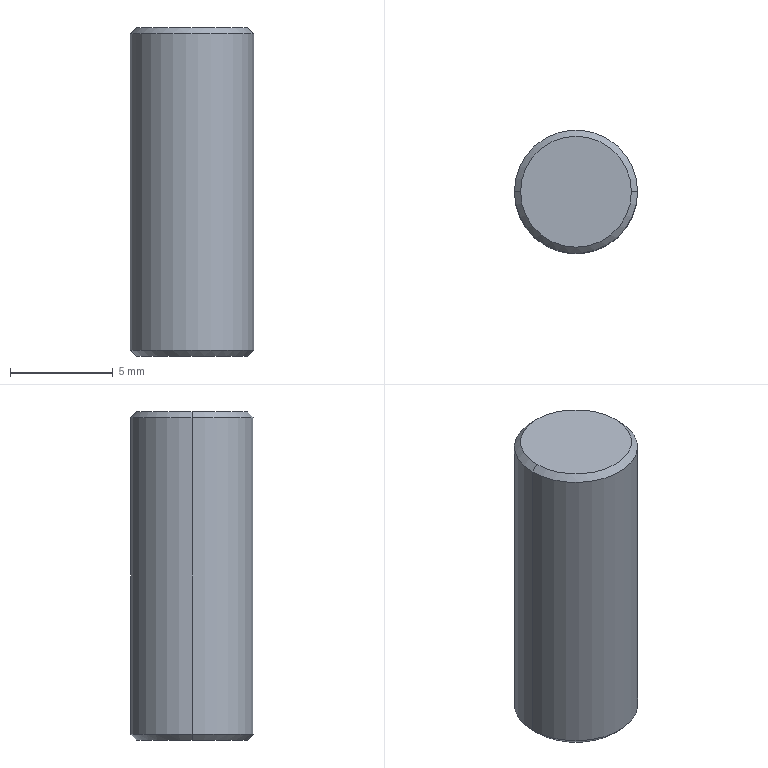Part | SolidWorks | features Chamfer 1, Extrusion 1 | 1 solid | 8 faces | box 6 x 6 x 16 mm | volume 450.749 mm3 | cone 4 | cylinder 2 | plane 2 | commonest cylinder face diameters 6 x2
STEP:
#1=CARTESIAN_POINT('',(2.7,0.,8.));
#2=VERTEX_POINT('',#1);
#3=CARTESIAN_POINT('',(-2.7,0.,8.));
#4=VERTEX_POINT('',#3);
#5=CARTESIAN_POINT('',(0.,0.,8.));
#6=DIRECTION('',(0.,0.,1.));
#7=DIRECTION('',(1.,0.,0.));
#8=AXIS2_PLACEMENT_3D('',#5,#6,#7);
#9=CIRCLE('',#8,2.7);
#10=EDGE_CURVE('',#2,#4,#9,.T.);
#11=ORIENTED_EDGE('',*,*,#10,.F.);
#12=CARTESIAN_POINT('',(3.,0.,7.7));
#13=VERTEX_POINT('',#12);
#14=CARTESIAN_POINT('',(2.7,0.,8.));
#15=DIRECTION('',(0.7071,0.,-0.7071));
#16=VECTOR('',#15,1000.);
#17=LINE('',#14,#16);
#18=EDGE_CURVE('',#2,#13,#17,.T.);
#19=ORIENTED_EDGE('',*,*,#18,.T.);
#20=CARTESIAN_POINT('',(-3.,0.,7.7));
#21=VERTEX_POINT('',#20);
#22=CARTESIAN_POINT('',(0.,0.,7.7));
#23=DIRECTION('',(0.,0.,-1.));
#24=DIRECTION('',(1.,0.,0.));
#25=AXIS2_PLACEMENT_3D('',#22,#23,#24);
#26=CIRCLE('',#25,3.);
#27=EDGE_CURVE('',#21,#13,#26,.T.);
#28=ORIENTED_EDGE('',*,*,#27,.F.);
#29=CARTESIAN_POINT('',(-2.7,0.,8.));
#30=DIRECTION('',(-0.7071,0.,-0.7071));
#31=VECTOR('',#30,1000.);
#32=LINE('',#29,#31);
#33=EDGE_CURVE('',#4,#21,#32,.T.);
#34=ORIENTED_EDGE('',*,*,#33,.F.);
#35=EDGE_LOOP('',(#11,#19,#28,#34));
#36=FACE_OUTER_BOUND('',#35,.T.);
#37=CARTESIAN_POINT('',(0.,0.,8.));
#38=DIRECTION('',(0.,0.,-1.));
#39=DIRECTION('',(-1.,0.,0.));
#40=AXIS2_PLACEMENT_3D('',#37,#38,#39);
#41=CONICAL_SURFACE('',#40,2.7,0.7854);
#42=ADVANCED_FACE('',(#36),#41,.T.);
#43=CARTESIAN_POINT('',(-2.7,0.,-8.));
#44=VERTEX_POINT('',#43);
#45=CARTESIAN_POINT('',(2.7,0.,-8.));
#46=VERTEX_POINT('',#45);
#47=CARTESIAN_POINT('',(0.,0.,-8.));
#48=DIRECTION('',(0.,0.,-1.));
#49=DIRECTION('',(1.,0.,0.));
#50=AXIS2_PLACEMENT_3D('',#47,#48,#49);
#51=CIRCLE('',#50,2.7);
#52=EDGE_CURVE('',#44,#46,#51,.T.);
#53=ORIENTED_EDGE('',*,*,#52,.F.);
#54=CARTESIAN_POINT('',(-3.,0.,-7.7));
#55=VERTEX_POINT('',#54);
#56=CARTESIAN_POINT('',(-3.,0.,-7.7));
#57=DIRECTION('',(-0.7071,0.,0.7071));
#58=VECTOR('',#57,1000.);
#59=LINE('',#56,#58);
#60=EDGE_CURVE('',#44,#55,#59,.T.);
#61=ORIENTED_EDGE('',*,*,#60,.T.);
#62=CARTESIAN_POINT('',(3.,0.,-7.7));
#63=VERTEX_POINT('',#62);
#64=CARTESIAN_POINT('',(0.,0.,-7.7));
#65=DIRECTION('',(0.,0.,1.));
#66=DIRECTION('',(1.,0.,0.));
#67=AXIS2_PLACEMENT_3D('',#64,#65,#66);
#68=CIRCLE('',#67,3.);
#69=EDGE_CURVE('',#63,#55,#68,.T.);
#70=ORIENTED_EDGE('',*,*,#69,.F.);
#71=CARTESIAN_POINT('',(3.,0.,-7.7));
#72=DIRECTION('',(0.7071,0.,0.7071));
#73=VECTOR('',#72,1000.);
#74=LINE('',#71,#73);
#75=EDGE_CURVE('',#46,#63,#74,.T.);
#76=ORIENTED_EDGE('',*,*,#75,.F.);
#77=EDGE_LOOP('',(#53,#61,#70,#76));
#78=FACE_OUTER_BOUND('',#77,.T.);
#79=CARTESIAN_POINT('',(0.,0.,-7.7));
#80=DIRECTION('',(0.,0.,1.));
#81=DIRECTION('',(1.,0.,0.));
#82=AXIS2_PLACEMENT_3D('',#79,#80,#81);
#83=CONICAL_SURFACE('',#82,3.,0.7854);
#84=ADVANCED_FACE('',(#78),#83,.T.);
#85=ORIENTED_EDGE('',*,*,#27,.T.);
#86=CARTESIAN_POINT('',(3.,0.,8.));
#87=DIRECTION('',(0.,0.,-1.));
#88=VECTOR('',#87,1000.);
#89=LINE('',#86,#88);
#90=EDGE_CURVE('',#13,#63,#89,.T.);
#91=ORIENTED_EDGE('',*,*,#90,.T.);
#92=ORIENTED_EDGE('',*,*,#69,.T.);
#93=CARTESIAN_POINT('',(-3.,0.,8.));
#94=DIRECTION('',(0.,0.,-1.));
#95=VECTOR('',#94,1000.);
#96=LINE('',#93,#95);
#97=EDGE_CURVE('',#21,#55,#96,.T.);
#98=ORIENTED_EDGE('',*,*,#97,.F.);
#99=EDGE_LOOP('',(#85,#91,#92,#98));
#100=FACE_OUTER_BOUND('',#99,.T.);
#101=CARTESIAN_POINT('',(0.,0.,8.));
#102=DIRECTION('',(0.,0.,-1.));
#103=DIRECTION('',(-1.,0.,0.));
#104=AXIS2_PLACEMENT_3D('',#101,#102,#103);
#105=CYLINDRICAL_SURFACE('',#104,3.);
#106=ADVANCED_FACE('',(#100),#105,.T.);
#107=ORIENTED_EDGE('',*,*,#90,.F.);
#108=CARTESIAN_POINT('',(0.,0.,7.7));
#109=DIRECTION('',(0.,0.,-1.));
#110=DIRECTION('',(1.,0.,0.));
#111=AXIS2_PLACEMENT_3D('',#108,#109,#110);
#112=CIRCLE('',#111,3.);
#113=EDGE_CURVE('',#13,#21,#112,.T.);
#114=ORIENTED_EDGE('',*,*,#113,.T.);
#115=ORIENTED_EDGE('',*,*,#97,.T.);
#116=CARTESIAN_POINT('',(0.,0.,-7.7));
#117=DIRECTION('',(0.,0.,1.));
#118=DIRECTION('',(1.,0.,0.));
#119=AXIS2_PLACEMENT_3D('',#116,#117,#118);
#120=CIRCLE('',#119,3.);
#121=EDGE_CURVE('',#55,#63,#120,.T.);
#122=ORIENTED_EDGE('',*,*,#121,.T.);
#123=EDGE_LOOP('',(#107,#114,#115,#122));
#124=FACE_OUTER_BOUND('',#123,.T.);
#125=CARTESIAN_POINT('',(0.,0.,8.));
#126=DIRECTION('',(0.,0.,-1.));
#127=DIRECTION('',(-1.,0.,0.));
#128=AXIS2_PLACEMENT_3D('',#125,#126,#127);
#129=CYLINDRICAL_SURFACE('',#128,3.);
#130=ADVANCED_FACE('',(#124),#129,.T.);
#131=CARTESIAN_POINT('',(0.,0.,8.));
#132=DIRECTION('',(0.,0.,1.));
#133=DIRECTION('',(1.,0.,0.));
#134=AXIS2_PLACEMENT_3D('',#131,#132,#133);
#135=CIRCLE('',#134,2.7);
#136=EDGE_CURVE('',#4,#2,#135,.T.);
#137=ORIENTED_EDGE('',*,*,#136,.T.);
#138=ORIENTED_EDGE('',*,*,#10,.T.);
#139=EDGE_LOOP('',(#137,#138));
#140=FACE_OUTER_BOUND('',#139,.T.);
#141=CARTESIAN_POINT('',(0.,0.,8.));
#142=DIRECTION('',(0.,0.,1.));
#143=DIRECTION('',(1.,0.,0.));
#144=AXIS2_PLACEMENT_3D('',#141,#142,#143);
#145=PLANE('',#144);
#146=ADVANCED_FACE('',(#140),#145,.T.);
#147=CARTESIAN_POINT('',(0.,0.,-8.));
#148=DIRECTION('',(0.,0.,-1.));
#149=DIRECTION('',(1.,0.,0.));
#150=AXIS2_PLACEMENT_3D('',#147,#148,#149);
#151=CIRCLE('',#150,2.7);
#152=EDGE_CURVE('',#46,#44,#151,.T.);
#153=ORIENTED_EDGE('',*,*,#152,.T.);
#154=ORIENTED_EDGE('',*,*,#52,.T.);
#155=EDGE_LOOP('',(#153,#154));
#156=FACE_OUTER_BOUND('',#155,.T.);
#157=CARTESIAN_POINT('',(0.,0.,-8.));
#158=DIRECTION('',(0.,0.,1.));
#159=DIRECTION('',(1.,0.,0.));
#160=AXIS2_PLACEMENT_3D('',#157,#158,#159);
#161=PLANE('',#160);
#162=ADVANCED_FACE('',(#156),#161,.F.);
#163=ORIENTED_EDGE('',*,*,#60,.F.);
#164=ORIENTED_EDGE('',*,*,#152,.F.);
#165=ORIENTED_EDGE('',*,*,#75,.T.);
#166=ORIENTED_EDGE('',*,*,#121,.F.);
#167=EDGE_LOOP('',(#163,#164,#165,#166));
#168=FACE_OUTER_BOUND('',#167,.T.);
#169=CARTESIAN_POINT('',(0.,0.,-7.7));
#170=DIRECTION('',(0.,0.,1.));
#171=DIRECTION('',(1.,0.,0.));
#172=AXIS2_PLACEMENT_3D('',#169,#170,#171);
#173=CONICAL_SURFACE('',#172,3.,0.7854);
#174=ADVANCED_FACE('',(#168),#173,.T.);
#175=ORIENTED_EDGE('',*,*,#18,.F.);
#176=ORIENTED_EDGE('',*,*,#136,.F.);
#177=ORIENTED_EDGE('',*,*,#33,.T.);
#178=ORIENTED_EDGE('',*,*,#113,.F.);
#179=EDGE_LOOP('',(#175,#176,#177,#178));
#180=FACE_OUTER_BOUND('',#179,.T.);
#181=CARTESIAN_POINT('',(0.,0.,8.));
#182=DIRECTION('',(0.,0.,-1.));
#183=DIRECTION('',(-1.,0.,0.));
#184=AXIS2_PLACEMENT_3D('',#181,#182,#183);
#185=CONICAL_SURFACE('',#184,2.7,0.7854);
#186=ADVANCED_FACE('',(#180),#185,.T.);
#187=CLOSED_SHELL('',(#42,#84,#106,#130,#146,#162,#174,#186));
#188=MANIFOLD_SOLID_BREP('',#187);
#189=CARTESIAN_POINT('',(0.,0.,0.));
#190=DIRECTION('',(0.,0.,1.));
#191=DIRECTION('',(1.,0.,0.));
#192=AXIS2_PLACEMENT_3D('',#189,#190,#191);
#193=(LENGTH_UNIT()NAMED_UNIT(*)SI_UNIT(.MILLI.,.METRE.));
#194=UNCERTAINTY_MEASURE_WITH_UNIT(LENGTH_MEASURE(0.00001),#193,'','');
#195=(NAMED_UNIT(*)PLANE_ANGLE_UNIT()SI_UNIT($,.RADIAN.));
#196=(NAMED_UNIT(*)SI_UNIT($,.STERADIAN.)SOLID_ANGLE_UNIT());
#197=(GEOMETRIC_REPRESENTATION_CONTEXT(3)GLOBAL_UNCERTAINTY_ASSIGNED_CONTEXT((#194))GLOBAL_UNIT_ASSIGNED_CONTEXT((#193,#195,#196))REPRESENTATION_CONTEXT('',''));
#198=ADVANCED_BREP_SHAPE_REPRESENTATION('',(#188,#192),#197);